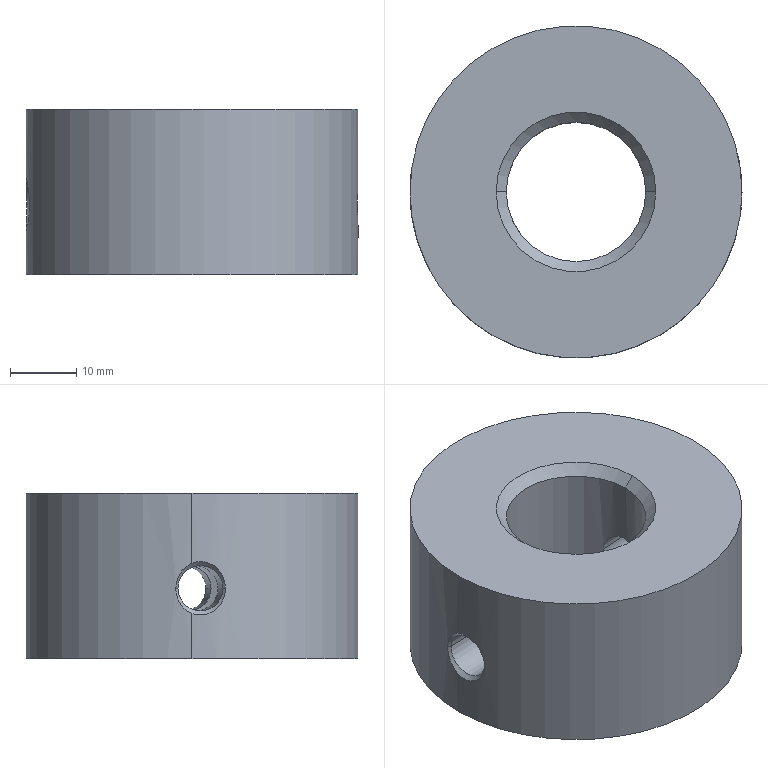Part | SolidWorks | features 3DProfileFeature 2, HoleWzd 2, Extrusion 1 | 1 solid | 14 faces | box 50 x 50 x 25 mm | volume 39286 mm3 | cylinder 8 | cone 4 | plane 2 | commonest cylinder face diameters 6.8 x4 21 x2 50 x2
STEP:
#1=CARTESIAN_POINT('',(24.555,4.697,10.643));
#2=VERTEX_POINT('',#1);
#3=CARTESIAN_POINT('',(25.,0.,7.507));
#4=VERTEX_POINT('',#3);
#5=CARTESIAN_POINT('',(24.555,4.697,10.643));
#6=CARTESIAN_POINT('',(24.555,4.697,10.365));
#7=CARTESIAN_POINT('',(24.561,4.663,10.087));
#8=CARTESIAN_POINT('',(24.587,4.527,9.543));
#9=CARTESIAN_POINT('',(24.605,4.428,9.284));
#10=CARTESIAN_POINT('',(24.639,4.232,8.916));
#11=CARTESIAN_POINT('',(24.652,4.158,8.796));
#12=CARTESIAN_POINT('',(24.678,3.999,8.568));
#13=CARTESIAN_POINT('',(24.692,3.913,8.46));
#14=CARTESIAN_POINT('',(24.735,3.635,8.152));
#15=CARTESIAN_POINT('',(24.766,3.421,7.967));
#16=CARTESIAN_POINT('',(24.825,2.961,7.659));
#17=CARTESIAN_POINT('',(24.854,2.715,7.535));
#18=CARTESIAN_POINT('',(24.906,2.186,7.346));
#19=CARTESIAN_POINT('',(24.928,1.916,7.286));
#20=CARTESIAN_POINT('',(24.964,1.363,7.232));
#21=CARTESIAN_POINT('',(24.978,1.079,7.24));
#22=CARTESIAN_POINT('',(24.991,0.6674,7.303));
#23=CARTESIAN_POINT('',(24.995,0.5315,7.332));
#24=CARTESIAN_POINT('',(24.999,0.2625,7.407));
#25=CARTESIAN_POINT('',(25.,0.1288,7.454));
#26=CARTESIAN_POINT('',(25.,0.,7.507));
#27=B_SPLINE_CURVE_WITH_KNOTS('',3,(#5,#6,#7,#8,#9,#10,#11,#12,#13,#14,#15,#16,#17,#18,#19,#20,#21,#22,#23,#24,#25,#26),.UNSPECIFIED.,.F.,.F.,(4,2,2,2,2,2,2,2,2,2,4),(0.01064,0.01148,0.01231,0.01272,0.01314,0.01397,0.01481,0.01564,0.01647,0.01689,0.01731),.UNSPECIFIED.);
#28=EDGE_CURVE('',#2,#4,#27,.T.);
#29=ORIENTED_EDGE('',*,*,#28,.F.);
#30=CARTESIAN_POINT('',(9.742,3.917,10.643));
#31=VERTEX_POINT('',#30);
#32=CARTESIAN_POINT('',(-25.144,2.082,10.643));
#33=DIRECTION('',(-0.9986,-0.05254,0.));
#34=VECTOR('',#33,1000.);
#35=LINE('',#32,#34);
#36=EDGE_CURVE('',#2,#31,#35,.T.);
#37=ORIENTED_EDGE('',*,*,#36,.T.);
#38=CARTESIAN_POINT('',(10.5,0.,7.288));
#39=VERTEX_POINT('',#38);
#40=CARTESIAN_POINT('',(10.5,0.,7.288));
#41=CARTESIAN_POINT('',(10.5,0.2463,7.248));
#42=CARTESIAN_POINT('',(10.491,0.4921,7.235));
#43=CARTESIAN_POINT('',(10.457,0.9829,7.262));
#44=CARTESIAN_POINT('',(10.43,1.23,7.303));
#45=CARTESIAN_POINT('',(10.364,1.7,7.436));
#46=CARTESIAN_POINT('',(10.324,1.926,7.527));
#47=CARTESIAN_POINT('',(10.234,2.358,7.759));
#48=CARTESIAN_POINT('',(10.186,2.557,7.896));
#49=CARTESIAN_POINT('',(10.087,2.923,8.212));
#50=CARTESIAN_POINT('',(10.036,3.091,8.392));
#51=CARTESIAN_POINT('',(9.942,3.381,8.779));
#52=CARTESIAN_POINT('',(9.899,3.504,8.987));
#53=CARTESIAN_POINT('',(9.824,3.709,9.435));
#54=CARTESIAN_POINT('',(9.794,3.786,9.668));
#55=CARTESIAN_POINT('',(9.753,3.89,10.147));
#56=CARTESIAN_POINT('',(9.742,3.917,10.397));
#57=CARTESIAN_POINT('',(9.742,3.917,10.643));
#58=B_SPLINE_CURVE_WITH_KNOTS('',3,(#40,#41,#42,#43,#44,#45,#46,#47,#48,#49,#50,#51,#52,#53,#54,#55,#56,#57),.UNSPECIFIED.,.F.,.F.,(4,2,2,2,2,2,2,2,4),(0.,0.0007379,0.001476,0.002214,0.002952,0.00369,0.004427,0.005165,0.005903),.UNSPECIFIED.);
#59=EDGE_CURVE('',#39,#31,#58,.T.);
#60=ORIENTED_EDGE('',*,*,#59,.F.);
#61=CARTESIAN_POINT('',(10.099,-2.873,10.643));
#62=VERTEX_POINT('',#61);
#63=CARTESIAN_POINT('',(10.099,-2.873,10.643));
#64=CARTESIAN_POINT('',(10.099,-2.873,10.443));
#65=CARTESIAN_POINT('',(10.105,-2.855,10.239));
#66=CARTESIAN_POINT('',(10.125,-2.783,9.845));
#67=CARTESIAN_POINT('',(10.139,-2.73,9.653));
#68=CARTESIAN_POINT('',(10.176,-2.589,9.277));
#69=CARTESIAN_POINT('',(10.198,-2.501,9.095));
#70=CARTESIAN_POINT('',(10.246,-2.298,8.753));
#71=CARTESIAN_POINT('',(10.272,-2.182,8.592));
#72=CARTESIAN_POINT('',(10.324,-1.92,8.288));
#73=CARTESIAN_POINT('',(10.35,-1.776,8.148));
#74=CARTESIAN_POINT('',(10.398,-1.469,7.897));
#75=CARTESIAN_POINT('',(10.42,-1.305,7.784));
#76=CARTESIAN_POINT('',(10.477,-0.7779,7.488));
#77=CARTESIAN_POINT('',(10.5,-0.4003,7.354));
#78=CARTESIAN_POINT('',(10.5,0.,7.288));
#79=B_SPLINE_CURVE_WITH_KNOTS('',3,(#63,#64,#65,#66,#67,#68,#69,#70,#71,#72,#73,#74,#75,#76,#77,#78),.UNSPECIFIED.,.F.,.F.,(4,2,2,2,2,2,2,4),(0.01661,0.01721,0.01781,0.01841,0.01901,0.01961,0.02021,0.02141),.UNSPECIFIED.);
#80=EDGE_CURVE('',#62,#39,#79,.T.);
#81=ORIENTED_EDGE('',*,*,#80,.F.);
#82=CARTESIAN_POINT('',(24.912,-2.094,10.643));
#83=VERTEX_POINT('',#82);
#84=CARTESIAN_POINT('',(-24.787,-4.709,10.643));
#85=DIRECTION('',(-0.9986,-0.05254,0.));
#86=VECTOR('',#85,1000.);
#87=LINE('',#84,#86);
#88=EDGE_CURVE('',#83,#62,#87,.T.);
#89=ORIENTED_EDGE('',*,*,#88,.F.);
#90=CARTESIAN_POINT('',(25.,0.,7.507));
#91=CARTESIAN_POINT('',(25.,-0.3073,7.636));
#92=CARTESIAN_POINT('',(24.994,-0.5936,7.808));
#93=CARTESIAN_POINT('',(24.977,-1.111,8.233));
#94=CARTESIAN_POINT('',(24.965,-1.333,8.479));
#95=CARTESIAN_POINT('',(24.942,-1.706,9.035));
#96=CARTESIAN_POINT('',(24.932,-1.849,9.336));
#97=CARTESIAN_POINT('',(24.92,-1.995,9.814));
#98=CARTESIAN_POINT('',(24.917,-2.032,9.978));
#99=CARTESIAN_POINT('',(24.913,-2.082,10.309));
#100=CARTESIAN_POINT('',(24.912,-2.094,10.475));
#101=CARTESIAN_POINT('',(24.912,-2.094,10.643));
#102=B_SPLINE_CURVE_WITH_KNOTS('',3,(#90,#91,#92,#93,#94,#95,#96,#97,#98,#99,#100,#101),.UNSPECIFIED.,.F.,.F.,(4,2,2,2,2,4),(0.01731,0.0183,0.01929,0.02029,0.02078,0.02128),.UNSPECIFIED.);
#103=EDGE_CURVE('',#4,#83,#102,.T.);
#104=ORIENTED_EDGE('',*,*,#103,.F.);
#105=EDGE_LOOP('',(#29,#37,#60,#81,#89,#104));
#106=FACE_OUTER_BOUND('',#105,.T.);
#107=CARTESIAN_POINT('',(-24.965,-1.314,10.643));
#108=DIRECTION('',(-0.9986,-0.05254,0.));
#109=DIRECTION('',(0.05254,-0.9986,0.));
#110=AXIS2_PLACEMENT_3D('',#107,#108,#109);
#111=CYLINDRICAL_SURFACE('',#110,3.4);
#112=ADVANCED_FACE('',(#106),#111,.F.);
#113=CARTESIAN_POINT('',(-10.099,2.873,10.643));
#114=VERTEX_POINT('',#113);
#115=CARTESIAN_POINT('',(-10.5,0.,7.288));
#116=VERTEX_POINT('',#115);
#117=CARTESIAN_POINT('',(-10.099,2.873,10.643));
#118=CARTESIAN_POINT('',(-10.099,2.873,10.244));
#119=CARTESIAN_POINT('',(-10.121,2.799,9.839));
#120=CARTESIAN_POINT('',(-10.176,2.589,9.278));
#121=CARTESIAN_POINT('',(-10.198,2.502,9.096));
#122=CARTESIAN_POINT('',(-10.246,2.297,8.752));
#123=CARTESIAN_POINT('',(-10.272,2.181,8.591));
#124=CARTESIAN_POINT('',(-10.324,1.921,8.289));
#125=CARTESIAN_POINT('',(-10.35,1.777,8.148));
#126=CARTESIAN_POINT('',(-10.398,1.467,7.895));
#127=CARTESIAN_POINT('',(-10.42,1.303,7.783));
#128=CARTESIAN_POINT('',(-10.458,0.9555,7.588));
#129=CARTESIAN_POINT('',(-10.473,0.7699,7.503));
#130=CARTESIAN_POINT('',(-10.494,0.3914,7.37));
#131=CARTESIAN_POINT('',(-10.5,0.1978,7.321));
#132=CARTESIAN_POINT('',(-10.5,0.,7.288));
#133=B_SPLINE_CURVE_WITH_KNOTS('',3,(#117,#118,#119,#120,#121,#122,#123,#124,#125,#126,#127,#128,#129,#130,#131,#132),.UNSPECIFIED.,.F.,.F.,(4,2,2,2,2,2,2,4),(0.0107,0.0119,0.0125,0.0131,0.0137,0.0143,0.0149,0.0155),.UNSPECIFIED.);
#134=EDGE_CURVE('',#114,#116,#133,.T.);
#135=ORIENTED_EDGE('',*,*,#134,.F.);
#136=CARTESIAN_POINT('',(-24.52,2.115,10.643));
#137=VERTEX_POINT('',#136);
#138=CARTESIAN_POINT('',(-25.144,2.082,10.643));
#139=DIRECTION('',(-0.9986,-0.05254,0.));
#140=VECTOR('',#139,1000.);
#141=LINE('',#138,#140);
#142=EDGE_CURVE('',#114,#137,#141,.T.);
#143=ORIENTED_EDGE('',*,*,#142,.T.);
#144=CARTESIAN_POINT('',(-24.163,-4.676,10.643));
#145=VERTEX_POINT('',#144);
#146=CARTESIAN_POINT('',(-24.341,-1.281,10.643));
#147=DIRECTION('',(-0.9986,-0.05254,0.));
#148=DIRECTION('',(0.05254,-0.9986,0.));
#149=AXIS2_PLACEMENT_3D('',#146,#147,#148);
#150=CIRCLE('',#149,3.4);
#151=EDGE_CURVE('',#137,#145,#150,.T.);
#152=ORIENTED_EDGE('',*,*,#151,.T.);
#153=CARTESIAN_POINT('',(-9.742,-3.917,10.643));
#154=VERTEX_POINT('',#153);
#155=CARTESIAN_POINT('',(-24.787,-4.709,10.643));
#156=DIRECTION('',(-0.9986,-0.05254,0.));
#157=VECTOR('',#156,1000.);
#158=LINE('',#155,#157);
#159=EDGE_CURVE('',#154,#145,#158,.T.);
#160=ORIENTED_EDGE('',*,*,#159,.F.);
#161=CARTESIAN_POINT('',(-10.5,0.,7.288));
#162=CARTESIAN_POINT('',(-10.5,-0.2432,7.249));
#163=CARTESIAN_POINT('',(-10.491,-0.4945,7.235));
#164=CARTESIAN_POINT('',(-10.457,-0.9847,7.262));
#165=CARTESIAN_POINT('',(-10.431,-1.228,7.303));
#166=CARTESIAN_POINT('',(-10.364,-1.703,7.436));
#167=CARTESIAN_POINT('',(-10.324,-1.928,7.528));
#168=CARTESIAN_POINT('',(-10.235,-2.355,7.758));
#169=CARTESIAN_POINT('',(-10.185,-2.558,7.897));
#170=CARTESIAN_POINT('',(-10.087,-2.924,8.213));
#171=CARTESIAN_POINT('',(-10.036,-3.089,8.39));
#172=CARTESIAN_POINT('',(-9.942,-3.382,8.781));
#173=CARTESIAN_POINT('',(-9.898,-3.505,8.989));
#174=CARTESIAN_POINT('',(-9.824,-3.708,9.432));
#175=CARTESIAN_POINT('',(-9.794,-3.787,9.669));
#176=CARTESIAN_POINT('',(-9.753,-3.891,10.149));
#177=CARTESIAN_POINT('',(-9.742,-3.917,10.394));
#178=CARTESIAN_POINT('',(-9.742,-3.917,10.643));
#179=B_SPLINE_CURVE_WITH_KNOTS('',3,(#161,#162,#163,#164,#165,#166,#167,#168,#169,#170,#171,#172,#173,#174,#175,#176,#177,#178),.UNSPECIFIED.,.F.,.F.,(4,2,2,2,2,2,2,2,4),(0.0155,0.01624,0.01698,0.01771,0.01845,0.01919,0.01993,0.02066,0.0214),.UNSPECIFIED.);
#180=EDGE_CURVE('',#116,#154,#179,.T.);
#181=ORIENTED_EDGE('',*,*,#180,.F.);
#182=EDGE_LOOP('',(#135,#143,#152,#160,#181));
#183=FACE_OUTER_BOUND('',#182,.T.);
#184=CARTESIAN_POINT('',(-24.965,-1.314,10.643));
#185=DIRECTION('',(-0.9986,-0.05254,0.));
#186=DIRECTION('',(0.05254,-0.9986,0.));
#187=AXIS2_PLACEMENT_3D('',#184,#185,#186);
#188=CYLINDRICAL_SURFACE('',#187,3.4);
#189=ADVANCED_FACE('',(#183),#188,.F.);
#190=ORIENTED_EDGE('',*,*,#151,.F.);
#191=CARTESIAN_POINT('',(-24.881,2.439,10.643));
#192=VERTEX_POINT('',#191);
#193=CARTESIAN_POINT('',(-25.177,2.706,10.643));
#194=DIRECTION('',(-0.7433,0.669,0.));
#195=VECTOR('',#194,1000.);
#196=LINE('',#193,#195);
#197=EDGE_CURVE('',#137,#192,#196,.T.);
#198=ORIENTED_EDGE('',*,*,#197,.T.);
#199=CARTESIAN_POINT('',(-25.,0.,6.875));
#200=VERTEX_POINT('',#199);
#201=CARTESIAN_POINT('',(-25.,0.,6.875));
#202=CARTESIAN_POINT('',(-25.,0.1848,6.95));
#203=CARTESIAN_POINT('',(-24.998,0.3615,7.039));
#204=CARTESIAN_POINT('',(-24.991,0.6998,7.245));
#205=CARTESIAN_POINT('',(-24.986,0.8625,7.363));
#206=CARTESIAN_POINT('',(-24.973,1.166,7.621));
#207=CARTESIAN_POINT('',(-24.966,1.306,7.76));
#208=CARTESIAN_POINT('',(-24.951,1.565,8.059));
#209=CARTESIAN_POINT('',(-24.943,1.684,8.22));
#210=CARTESIAN_POINT('',(-24.92,2.004,8.725));
#211=CARTESIAN_POINT('',(-24.906,2.165,9.085));
#212=CARTESIAN_POINT('',(-24.886,2.385,9.855));
#213=CARTESIAN_POINT('',(-24.881,2.439,10.246));
#214=CARTESIAN_POINT('',(-24.881,2.439,10.643));
#215=B_SPLINE_CURVE_WITH_KNOTS('',3,(#201,#202,#203,#204,#205,#206,#207,#208,#209,#210,#211,#212,#213,#214),.UNSPECIFIED.,.F.,.F.,(4,2,2,2,2,2,4),(0.003713,0.004306,0.004899,0.005493,0.006086,0.007273,0.00846),.UNSPECIFIED.);
#216=EDGE_CURVE('',#200,#192,#215,.T.);
#217=ORIENTED_EDGE('',*,*,#216,.F.);
#218=CARTESIAN_POINT('',(-24.487,-5.037,10.643));
#219=VERTEX_POINT('',#218);
#220=CARTESIAN_POINT('',(-24.487,-5.037,10.643));
#221=CARTESIAN_POINT('',(-24.487,-5.037,10.333));
#222=CARTESIAN_POINT('',(-24.494,-5.004,10.026));
#223=CARTESIAN_POINT('',(-24.514,-4.905,9.57));
#224=CARTESIAN_POINT('',(-24.522,-4.863,9.419));
#225=CARTESIAN_POINT('',(-24.542,-4.764,9.124));
#226=CARTESIAN_POINT('',(-24.553,-4.707,8.981));
#227=CARTESIAN_POINT('',(-24.577,-4.578,8.702));
#228=CARTESIAN_POINT('',(-24.591,-4.506,8.566));
#229=CARTESIAN_POINT('',(-24.62,-4.345,8.301));
#230=CARTESIAN_POINT('',(-24.635,-4.256,8.172));
#231=CARTESIAN_POINT('',(-24.683,-3.971,7.805));
#232=CARTESIAN_POINT('',(-24.718,-3.754,7.586));
#233=CARTESIAN_POINT('',(-24.787,-3.265,7.199));
#234=CARTESIAN_POINT('',(-24.821,-3.001,7.04));
#235=CARTESIAN_POINT('',(-24.867,-2.576,6.853));
#236=CARTESIAN_POINT('',(-24.882,-2.429,6.799));
#237=CARTESIAN_POINT('',(-24.909,-2.132,6.713));
#238=CARTESIAN_POINT('',(-24.922,-1.981,6.68));
#239=CARTESIAN_POINT('',(-24.955,-1.524,6.611));
#240=CARTESIAN_POINT('',(-24.973,-1.208,6.606));
#241=CARTESIAN_POINT('',(-24.989,-0.7464,6.662));
#242=CARTESIAN_POINT('',(-24.993,-0.5945,6.69));
#243=CARTESIAN_POINT('',(-24.999,-0.2941,6.768));
#244=CARTESIAN_POINT('',(-25.,-0.1446,6.817));
#245=CARTESIAN_POINT('',(-25.,0.,6.875));
#246=B_SPLINE_CURVE_WITH_KNOTS('',3,(#220,#221,#222,#223,#224,#225,#226,#227,#228,#229,#230,#231,#232,#233,#234,#235,#236,#237,#238,#239,#240,#241,#242,#243,#244,#245),.UNSPECIFIED.,.F.,.F.,(4,2,2,2,2,2,2,2,2,2,2,2,4),(0.02064,0.02157,0.02203,0.0225,0.02296,0.02343,0.02435,0.02528,0.02575,0.02621,0.02714,0.02761,0.02807),.UNSPECIFIED.);
#247=EDGE_CURVE('',#219,#200,#246,.T.);
#248=ORIENTED_EDGE('',*,*,#247,.F.);
#249=CARTESIAN_POINT('',(-24.754,-5.333,10.643));
#250=DIRECTION('',(-0.669,-0.7433,0.));
#251=VECTOR('',#250,1000.);
#252=LINE('',#249,#251);
#253=EDGE_CURVE('',#145,#219,#252,.T.);
#254=ORIENTED_EDGE('',*,*,#253,.F.);
#255=EDGE_LOOP('',(#190,#198,#217,#248,#254));
#256=FACE_OUTER_BOUND('',#255,.T.);
#257=CARTESIAN_POINT('',(-24.965,-1.314,10.643));
#258=DIRECTION('',(-0.9986,-0.05254,0.));
#259=DIRECTION('',(0.05254,-0.9986,0.));
#260=AXIS2_PLACEMENT_3D('',#257,#258,#259);
#261=CONICAL_SURFACE('',#260,4.025,0.7854);
#262=ADVANCED_FACE('',(#256),#261,.F.);
#263=CARTESIAN_POINT('',(-10.5,0.,23.475));
#264=VERTEX_POINT('',#263);
#265=CARTESIAN_POINT('',(10.5,0.,23.475));
#266=VERTEX_POINT('',#265);
#267=CARTESIAN_POINT('',(0.,0.,23.475));
#268=DIRECTION('',(0.,0.,1.));
#269=DIRECTION('',(1.,0.,0.));
#270=AXIS2_PLACEMENT_3D('',#267,#268,#269);
#271=CIRCLE('',#270,10.5);
#272=EDGE_CURVE('',#264,#266,#271,.T.);
#273=ORIENTED_EDGE('',*,*,#272,.F.);
#274=CARTESIAN_POINT('',(-12.025,0.,25.));
#275=VERTEX_POINT('',#274);
#276=CARTESIAN_POINT('',(-12.025,0.,25.));
#277=DIRECTION('',(-0.7071,0.,0.7071));
#278=VECTOR('',#277,1000.);
#279=LINE('',#276,#278);
#280=EDGE_CURVE('',#264,#275,#279,.T.);
#281=ORIENTED_EDGE('',*,*,#280,.T.);
#282=CARTESIAN_POINT('',(12.025,0.,25.));
#283=VERTEX_POINT('',#282);
#284=CARTESIAN_POINT('',(0.,0.,25.));
#285=DIRECTION('',(0.,0.,1.));
#286=DIRECTION('',(1.,0.,0.));
#287=AXIS2_PLACEMENT_3D('',#284,#285,#286);
#288=CIRCLE('',#287,12.025);
#289=EDGE_CURVE('',#275,#283,#288,.T.);
#290=ORIENTED_EDGE('',*,*,#289,.T.);
#291=CARTESIAN_POINT('',(12.025,0.,25.));
#292=DIRECTION('',(0.7071,0.,0.7071));
#293=VECTOR('',#292,1000.);
#294=LINE('',#291,#293);
#295=EDGE_CURVE('',#266,#283,#294,.T.);
#296=ORIENTED_EDGE('',*,*,#295,.F.);
#297=EDGE_LOOP('',(#273,#281,#290,#296));
#298=FACE_OUTER_BOUND('',#297,.T.);
#299=CARTESIAN_POINT('',(0.,0.,25.));
#300=DIRECTION('',(0.,0.,1.));
#301=DIRECTION('',(1.,0.,0.));
#302=AXIS2_PLACEMENT_3D('',#299,#300,#301);
#303=CONICAL_SURFACE('',#302,12.025,0.7854);
#304=ADVANCED_FACE('',(#298),#303,.F.);
#305=CARTESIAN_POINT('',(-10.5,0.,0.));
#306=VERTEX_POINT('',#305);
#307=CARTESIAN_POINT('',(10.5,0.,0.));
#308=VERTEX_POINT('',#307);
#309=CARTESIAN_POINT('',(0.,0.,0.));
#310=DIRECTION('',(0.,0.,1.));
#311=DIRECTION('',(1.,0.,0.));
#312=AXIS2_PLACEMENT_3D('',#309,#310,#311);
#313=CIRCLE('',#312,10.5);
#314=EDGE_CURVE('',#306,#308,#313,.T.);
#315=ORIENTED_EDGE('',*,*,#314,.F.);
#316=CARTESIAN_POINT('',(-10.5,0.,25.));
#317=DIRECTION('',(0.,0.,1.));
#318=VECTOR('',#317,1000.);
#319=LINE('',#316,#318);
#320=EDGE_CURVE('',#306,#116,#319,.T.);
#321=ORIENTED_EDGE('',*,*,#320,.T.);
#322=ORIENTED_EDGE('',*,*,#180,.T.);
#323=CARTESIAN_POINT('',(-10.5,0.,13.998));
#324=VERTEX_POINT('',#323);
#325=CARTESIAN_POINT('',(-9.742,-3.917,10.643));
#326=CARTESIAN_POINT('',(-9.742,-3.917,10.893));
#327=CARTESIAN_POINT('',(-9.753,-3.891,11.138));
#328=CARTESIAN_POINT('',(-9.794,-3.787,11.617));
#329=CARTESIAN_POINT('',(-9.824,-3.708,11.855));
#330=CARTESIAN_POINT('',(-9.898,-3.505,12.298));
#331=CARTESIAN_POINT('',(-9.942,-3.382,12.507));
#332=CARTESIAN_POINT('',(-10.037,-3.088,12.899));
#333=CARTESIAN_POINT('',(-10.087,-2.923,13.075));
#334=CARTESIAN_POINT('',(-10.186,-2.557,13.39));
#335=CARTESIAN_POINT('',(-10.235,-2.354,13.53));
#336=CARTESIAN_POINT('',(-10.324,-1.927,13.759));
#337=CARTESIAN_POINT('',(-10.364,-1.702,13.851));
#338=CARTESIAN_POINT('',(-10.431,-1.229,13.984));
#339=CARTESIAN_POINT('',(-10.457,-0.9844,14.025));
#340=CARTESIAN_POINT('',(-10.491,-0.4947,14.052));
#341=CARTESIAN_POINT('',(-10.5,-0.2439,14.038));
#342=CARTESIAN_POINT('',(-10.5,0.,13.998));
#343=B_SPLINE_CURVE_WITH_KNOTS('',3,(#325,#326,#327,#328,#329,#330,#331,#332,#333,#334,#335,#336,#337,#338,#339,#340,#341,#342),.UNSPECIFIED.,.F.,.F.,(4,2,2,2,2,2,2,2,4),(0.,0.0007378,0.001476,0.002213,0.002951,0.003689,0.004427,0.005165,0.005902),.UNSPECIFIED.);
#344=EDGE_CURVE('',#154,#324,#343,.T.);
#345=ORIENTED_EDGE('',*,*,#344,.T.);
#346=CARTESIAN_POINT('',(-10.5,0.,25.));
#347=DIRECTION('',(0.,0.,1.));
#348=VECTOR('',#347,1000.);
#349=LINE('',#346,#348);
#350=EDGE_CURVE('',#324,#264,#349,.T.);
#351=ORIENTED_EDGE('',*,*,#350,.T.);
#352=ORIENTED_EDGE('',*,*,#272,.T.);
#353=CARTESIAN_POINT('',(10.5,0.,13.998));
#354=VERTEX_POINT('',#353);
#355=CARTESIAN_POINT('',(10.5,0.,25.));
#356=DIRECTION('',(0.,0.,1.));
#357=VECTOR('',#356,1000.);
#358=LINE('',#355,#357);
#359=EDGE_CURVE('',#354,#266,#358,.T.);
#360=ORIENTED_EDGE('',*,*,#359,.F.);
#361=CARTESIAN_POINT('',(10.5,0.,13.998));
#362=CARTESIAN_POINT('',(10.5,-0.1975,13.966));
#363=CARTESIAN_POINT('',(10.494,-0.3929,13.916));
#364=CARTESIAN_POINT('',(10.473,-0.7744,13.782));
#365=CARTESIAN_POINT('',(10.458,-0.9564,13.699));
#366=CARTESIAN_POINT('',(10.42,-1.304,13.503));
#367=CARTESIAN_POINT('',(10.398,-1.471,13.389));
#368=CARTESIAN_POINT('',(10.349,-1.781,13.135));
#369=CARTESIAN_POINT('',(10.323,-1.923,12.996));
#370=CARTESIAN_POINT('',(10.272,-2.182,12.695));
#371=CARTESIAN_POINT('',(10.246,-2.3,12.531));
#372=CARTESIAN_POINT('',(10.198,-2.504,12.187));
#373=CARTESIAN_POINT('',(10.176,-2.589,12.008));
#374=CARTESIAN_POINT('',(10.139,-2.729,11.634));
#375=CARTESIAN_POINT('',(10.124,-2.784,11.438));
#376=CARTESIAN_POINT('',(10.104,-2.855,11.043));
#377=CARTESIAN_POINT('',(10.099,-2.873,10.844));
#378=CARTESIAN_POINT('',(10.099,-2.873,10.643));
#379=B_SPLINE_CURVE_WITH_KNOTS('',3,(#361,#362,#363,#364,#365,#366,#367,#368,#369,#370,#371,#372,#373,#374,#375,#376,#377,#378),.UNSPECIFIED.,.F.,.F.,(4,2,2,2,2,2,2,2,4),(0.01181,0.01241,0.01301,0.01361,0.01421,0.01481,0.01541,0.01601,0.01661),.UNSPECIFIED.);
#380=EDGE_CURVE('',#354,#62,#379,.T.);
#381=ORIENTED_EDGE('',*,*,#380,.T.);
#382=ORIENTED_EDGE('',*,*,#80,.T.);
#383=CARTESIAN_POINT('',(10.5,0.,25.));
#384=DIRECTION('',(0.,0.,1.));
#385=VECTOR('',#384,1000.);
#386=LINE('',#383,#385);
#387=EDGE_CURVE('',#308,#39,#386,.T.);
#388=ORIENTED_EDGE('',*,*,#387,.F.);
#389=EDGE_LOOP('',(#315,#321,#322,#345,#351,#352,#360,#381,#382,#388));
#390=FACE_OUTER_BOUND('',#389,.T.);
#391=CARTESIAN_POINT('',(0.,0.,25.));
#392=DIRECTION('',(0.,0.,1.));
#393=DIRECTION('',(1.,0.,0.));
#394=AXIS2_PLACEMENT_3D('',#391,#392,#393);
#395=CYLINDRICAL_SURFACE('',#394,10.5);
#396=ADVANCED_FACE('',(#390),#395,.F.);
#397=CARTESIAN_POINT('',(25.,0.,25.));
#398=VERTEX_POINT('',#397);
#399=CARTESIAN_POINT('',(-25.,0.,25.));
#400=VERTEX_POINT('',#399);
#401=CARTESIAN_POINT('',(0.,0.,25.));
#402=DIRECTION('',(0.,0.,1.));
#403=DIRECTION('',(1.,0.,0.));
#404=AXIS2_PLACEMENT_3D('',#401,#402,#403);
#405=CIRCLE('',#404,25.);
#406=EDGE_CURVE('',#398,#400,#405,.T.);
#407=ORIENTED_EDGE('',*,*,#406,.F.);
#408=CARTESIAN_POINT('',(25.,0.,13.779));
#409=VERTEX_POINT('',#408);
#410=CARTESIAN_POINT('',(25.,0.,25.));
#411=DIRECTION('',(0.,0.,-1.));
#412=VECTOR('',#411,1000.);
#413=LINE('',#410,#412);
#414=EDGE_CURVE('',#398,#409,#413,.T.);
#415=ORIENTED_EDGE('',*,*,#414,.T.);
#416=CARTESIAN_POINT('',(25.,0.,13.779));
#417=CARTESIAN_POINT('',(25.,0.1281,13.833));
#418=CARTESIAN_POINT('',(24.999,0.2593,13.879));
#419=CARTESIAN_POINT('',(24.995,0.5285,13.954));
#420=CARTESIAN_POINT('',(24.991,0.6668,13.984));
#421=CARTESIAN_POINT('',(24.978,1.08,14.047));
#422=CARTESIAN_POINT('',(24.965,1.357,14.055));
#423=CARTESIAN_POINT('',(24.928,1.916,14.001));
#424=CARTESIAN_POINT('',(24.905,2.187,13.94));
#425=CARTESIAN_POINT('',(24.854,2.709,13.754));
#426=CARTESIAN_POINT('',(24.825,2.962,13.627));
#427=CARTESIAN_POINT('',(24.781,3.306,13.397));
#428=CARTESIAN_POINT('',(24.766,3.416,13.313));
#429=CARTESIAN_POINT('',(24.736,3.626,13.131));
#430=CARTESIAN_POINT('',(24.721,3.727,13.033));
#431=CARTESIAN_POINT('',(24.678,4.006,12.723));
#432=CARTESIAN_POINT('',(24.651,4.165,12.497));
#433=CARTESIAN_POINT('',(24.617,4.361,12.128));
#434=CARTESIAN_POINT('',(24.606,4.42,12.));
#435=CARTESIAN_POINT('',(24.588,4.519,11.74));
#436=CARTESIAN_POINT('',(24.58,4.561,11.608));
#437=CARTESIAN_POINT('',(24.562,4.662,11.204));
#438=CARTESIAN_POINT('',(24.555,4.697,10.921));
#439=CARTESIAN_POINT('',(24.555,4.697,10.643));
#440=B_SPLINE_CURVE_WITH_KNOTS('',3,(#416,#417,#418,#419,#420,#421,#422,#423,#424,#425,#426,#427,#428,#429,#430,#431,#432,#433,#434,#435,#436,#437,#438,#439),.UNSPECIFIED.,.F.,.F.,(4,2,2,2,2,2,2,2,2,2,2,4),(0.003979,0.004395,0.004812,0.005645,0.006478,0.00731,0.007727,0.008143,0.008976,0.009393,0.009809,0.01064),.UNSPECIFIED.);
#441=EDGE_CURVE('',#409,#2,#440,.T.);
#442=ORIENTED_EDGE('',*,*,#441,.T.);
#443=ORIENTED_EDGE('',*,*,#28,.T.);
#444=CARTESIAN_POINT('',(25.,0.,0.));
#445=VERTEX_POINT('',#444);
#446=CARTESIAN_POINT('',(25.,0.,25.));
#447=DIRECTION('',(0.,0.,-1.));
#448=VECTOR('',#447,1000.);
#449=LINE('',#446,#448);
#450=EDGE_CURVE('',#4,#445,#449,.T.);
#451=ORIENTED_EDGE('',*,*,#450,.T.);
#452=CARTESIAN_POINT('',(-25.,0.,0.));
#453=VERTEX_POINT('',#452);
#454=CARTESIAN_POINT('',(0.,0.,0.));
#455=DIRECTION('',(0.,0.,1.));
#456=DIRECTION('',(1.,0.,0.));
#457=AXIS2_PLACEMENT_3D('',#454,#455,#456);
#458=CIRCLE('',#457,25.);
#459=EDGE_CURVE('',#445,#453,#458,.T.);
#460=ORIENTED_EDGE('',*,*,#459,.T.);
#461=CARTESIAN_POINT('',(-25.,0.,25.));
#462=DIRECTION('',(0.,0.,-1.));
#463=VECTOR('',#462,1000.);
#464=LINE('',#461,#463);
#465=EDGE_CURVE('',#200,#453,#464,.T.);
#466=ORIENTED_EDGE('',*,*,#465,.F.);
#467=ORIENTED_EDGE('',*,*,#216,.T.);
#468=CARTESIAN_POINT('',(-25.,0.,14.412));
#469=VERTEX_POINT('',#468);
#470=CARTESIAN_POINT('',(-24.881,2.439,10.643));
#471=CARTESIAN_POINT('',(-24.881,2.439,10.842));
#472=CARTESIAN_POINT('',(-24.882,2.425,11.043));
#473=CARTESIAN_POINT('',(-24.887,2.37,11.435));
#474=CARTESIAN_POINT('',(-24.891,2.329,11.628));
#475=CARTESIAN_POINT('',(-24.901,2.22,12.008));
#476=CARTESIAN_POINT('',(-24.907,2.152,12.197));
#477=CARTESIAN_POINT('',(-24.921,1.989,12.56));
#478=CARTESIAN_POINT('',(-24.928,1.895,12.734));
#479=CARTESIAN_POINT('',(-24.943,1.684,13.067));
#480=CARTESIAN_POINT('',(-24.951,1.566,13.226));
#481=CARTESIAN_POINT('',(-24.966,1.305,13.528));
#482=CARTESIAN_POINT('',(-24.973,1.163,13.668));
#483=CARTESIAN_POINT('',(-24.986,0.8624,13.924));
#484=CARTESIAN_POINT('',(-24.991,0.7028,14.04));
#485=CARTESIAN_POINT('',(-24.998,0.3643,14.246));
#486=CARTESIAN_POINT('',(-25.,0.1838,14.337));
#487=CARTESIAN_POINT('',(-25.,0.,14.412));
#488=B_SPLINE_CURVE_WITH_KNOTS('',3,(#470,#471,#472,#473,#474,#475,#476,#477,#478,#479,#480,#481,#482,#483,#484,#485,#486,#487),.UNSPECIFIED.,.F.,.F.,(4,2,2,2,2,2,2,2,4),(0.00846,0.009054,0.009648,0.01024,0.01084,0.01143,0.01202,0.01262,0.01321),.UNSPECIFIED.);
#489=EDGE_CURVE('',#192,#469,#488,.T.);
#490=ORIENTED_EDGE('',*,*,#489,.T.);
#491=CARTESIAN_POINT('',(-25.,0.,25.));
#492=DIRECTION('',(0.,0.,-1.));
#493=VECTOR('',#492,1000.);
#494=LINE('',#491,#493);
#495=EDGE_CURVE('',#400,#469,#494,.T.);
#496=ORIENTED_EDGE('',*,*,#495,.F.);
#497=EDGE_LOOP('',(#407,#415,#442,#443,#451,#460,#466,#467,#490,#496));
#498=FACE_OUTER_BOUND('',#497,.T.);
#499=CARTESIAN_POINT('',(0.,0.,25.));
#500=DIRECTION('',(0.,0.,-1.));
#501=DIRECTION('',(-1.,0.,0.));
#502=AXIS2_PLACEMENT_3D('',#499,#500,#501);
#503=CYLINDRICAL_SURFACE('',#502,25.);
#504=ADVANCED_FACE('',(#498),#503,.T.);
#505=ORIENTED_EDGE('',*,*,#414,.F.);
#506=CARTESIAN_POINT('',(0.,0.,25.));
#507=DIRECTION('',(0.,0.,1.));
#508=DIRECTION('',(1.,0.,0.));
#509=AXIS2_PLACEMENT_3D('',#506,#507,#508);
#510=CIRCLE('',#509,25.);
#511=EDGE_CURVE('',#400,#398,#510,.T.);
#512=ORIENTED_EDGE('',*,*,#511,.F.);
#513=ORIENTED_EDGE('',*,*,#495,.T.);
#514=CARTESIAN_POINT('',(-25.,0.,14.412));
#515=CARTESIAN_POINT('',(-25.,-0.2874,14.528));
#516=CARTESIAN_POINT('',(-24.995,-0.5861,14.606));
#517=CARTESIAN_POINT('',(-24.973,-1.207,14.681));
#518=CARTESIAN_POINT('',(-24.956,-1.518,14.676));
#519=CARTESIAN_POINT('',(-24.922,-1.977,14.608));
#520=CARTESIAN_POINT('',(-24.91,-2.13,14.574));
#521=CARTESIAN_POINT('',(-24.882,-2.429,14.488));
#522=CARTESIAN_POINT('',(-24.868,-2.574,14.435));
#523=CARTESIAN_POINT('',(-24.821,-2.997,14.249));
#524=CARTESIAN_POINT('',(-24.787,-3.266,14.086));
#525=CARTESIAN_POINT('',(-24.718,-3.75,13.705));
#526=CARTESIAN_POINT('',(-24.684,-3.969,13.483));
#527=CARTESIAN_POINT('',(-24.619,-4.35,12.994));
#528=CARTESIAN_POINT('',(-24.59,-4.51,12.731));
#529=CARTESIAN_POINT('',(-24.553,-4.706,12.309));
#530=CARTESIAN_POINT('',(-24.542,-4.764,12.163));
#531=CARTESIAN_POINT('',(-24.523,-4.863,11.869));
#532=CARTESIAN_POINT('',(-24.514,-4.904,11.72));
#533=CARTESIAN_POINT('',(-24.501,-4.97,11.418));
#534=CARTESIAN_POINT('',(-24.496,-4.995,11.265));
#535=CARTESIAN_POINT('',(-24.489,-5.028,10.956));
#536=CARTESIAN_POINT('',(-24.487,-5.037,10.799));
#537=CARTESIAN_POINT('',(-24.487,-5.037,10.643));
#538=B_SPLINE_CURVE_WITH_KNOTS('',3,(#514,#515,#516,#517,#518,#519,#520,#521,#522,#523,#524,#525,#526,#527,#528,#529,#530,#531,#532,#533,#534,#535,#536,#537),.UNSPECIFIED.,.F.,.F.,(4,2,2,2,2,2,2,2,2,2,2,4),(0.01321,0.01414,0.01507,0.01553,0.016,0.01693,0.01785,0.01878,0.01925,0.01971,0.02018,0.02064),.UNSPECIFIED.);
#539=EDGE_CURVE('',#469,#219,#538,.T.);
#540=ORIENTED_EDGE('',*,*,#539,.T.);
#541=ORIENTED_EDGE('',*,*,#247,.T.);
#542=ORIENTED_EDGE('',*,*,#465,.T.);
#543=CARTESIAN_POINT('',(0.,0.,0.));
#544=DIRECTION('',(0.,0.,1.));
#545=DIRECTION('',(1.,0.,0.));
#546=AXIS2_PLACEMENT_3D('',#543,#544,#545);
#547=CIRCLE('',#546,25.);
#548=EDGE_CURVE('',#453,#445,#547,.T.);
#549=ORIENTED_EDGE('',*,*,#548,.T.);
#550=ORIENTED_EDGE('',*,*,#450,.F.);
#551=ORIENTED_EDGE('',*,*,#103,.T.);
#552=CARTESIAN_POINT('',(24.912,-2.094,10.643));
#553=CARTESIAN_POINT('',(24.912,-2.094,10.98));
#554=CARTESIAN_POINT('',(24.916,-2.045,11.308));
#555=CARTESIAN_POINT('',(24.928,-1.899,11.787));
#556=CARTESIAN_POINT('',(24.932,-1.838,11.945));
#557=CARTESIAN_POINT('',(24.943,-1.696,12.245));
#558=CARTESIAN_POINT('',(24.948,-1.614,12.389));
#559=CARTESIAN_POINT('',(24.959,-1.429,12.665));
#560=CARTESIAN_POINT('',(24.965,-1.325,12.798));
#561=CARTESIAN_POINT('',(24.976,-1.101,13.045));
#562=CARTESIAN_POINT('',(24.981,-0.9814,13.16));
#563=CARTESIAN_POINT('',(24.994,-0.5972,13.476));
#564=CARTESIAN_POINT('',(25.,-0.3058,13.652));
#565=CARTESIAN_POINT('',(25.,0.,13.779));
#566=B_SPLINE_CURVE_WITH_KNOTS('',3,(#552,#553,#554,#555,#556,#557,#558,#559,#560,#561,#562,#563,#564,#565),.UNSPECIFIED.,.F.,.F.,(4,2,2,2,2,2,4),(0.,0.0009947,0.001492,0.001989,0.002487,0.002984,0.003979),.UNSPECIFIED.);
#567=EDGE_CURVE('',#83,#409,#566,.T.);
#568=ORIENTED_EDGE('',*,*,#567,.T.);
#569=EDGE_LOOP('',(#505,#512,#513,#540,#541,#542,#549,#550,#551,#568));
#570=FACE_OUTER_BOUND('',#569,.T.);
#571=CARTESIAN_POINT('',(0.,0.,25.));
#572=DIRECTION('',(0.,0.,-1.));
#573=DIRECTION('',(-1.,0.,0.));
#574=AXIS2_PLACEMENT_3D('',#571,#572,#573);
#575=CYLINDRICAL_SURFACE('',#574,25.);
#576=ADVANCED_FACE('',(#570),#575,.T.);
#577=CARTESIAN_POINT('',(0.,0.,25.));
#578=DIRECTION('',(0.,0.,1.));
#579=DIRECTION('',(1.,0.,0.));
#580=AXIS2_PLACEMENT_3D('',#577,#578,#579);
#581=CIRCLE('',#580,12.025);
#582=EDGE_CURVE('',#283,#275,#581,.T.);
#583=ORIENTED_EDGE('',*,*,#582,.F.);
#584=ORIENTED_EDGE('',*,*,#289,.F.);
#585=EDGE_LOOP('',(#583,#584));
#586=FACE_BOUND('',#585,.T.);
#587=ORIENTED_EDGE('',*,*,#511,.T.);
#588=ORIENTED_EDGE('',*,*,#406,.T.);
#589=EDGE_LOOP('',(#587,#588));
#590=FACE_OUTER_BOUND('',#589,.T.);
#591=CARTESIAN_POINT('',(0.,0.,25.));
#592=DIRECTION('',(0.,0.,1.));
#593=DIRECTION('',(1.,0.,0.));
#594=AXIS2_PLACEMENT_3D('',#591,#592,#593);
#595=PLANE('',#594);
#596=ADVANCED_FACE('',(#586,#590),#595,.T.);
#597=CARTESIAN_POINT('',(0.,0.,0.));
#598=DIRECTION('',(0.,0.,1.));
#599=DIRECTION('',(1.,0.,0.));
#600=AXIS2_PLACEMENT_3D('',#597,#598,#599);
#601=CIRCLE('',#600,10.5);
#602=EDGE_CURVE('',#308,#306,#601,.T.);
#603=ORIENTED_EDGE('',*,*,#602,.T.);
#604=ORIENTED_EDGE('',*,*,#314,.T.);
#605=EDGE_LOOP('',(#603,#604));
#606=FACE_BOUND('',#605,.T.);
#607=ORIENTED_EDGE('',*,*,#548,.F.);
#608=ORIENTED_EDGE('',*,*,#459,.F.);
#609=EDGE_LOOP('',(#607,#608));
#610=FACE_OUTER_BOUND('',#609,.T.);
#611=CARTESIAN_POINT('',(0.,0.,0.));
#612=DIRECTION('',(0.,0.,1.));
#613=DIRECTION('',(1.,0.,0.));
#614=AXIS2_PLACEMENT_3D('',#611,#612,#613);
#615=PLANE('',#614);
#616=ADVANCED_FACE('',(#606,#610),#615,.F.);
#617=ORIENTED_EDGE('',*,*,#320,.F.);
#618=ORIENTED_EDGE('',*,*,#602,.F.);
#619=ORIENTED_EDGE('',*,*,#387,.T.);
#620=ORIENTED_EDGE('',*,*,#59,.T.);
#621=CARTESIAN_POINT('',(9.742,3.917,10.643));
#622=CARTESIAN_POINT('',(9.742,3.917,10.89));
#623=CARTESIAN_POINT('',(9.753,3.891,11.135));
#624=CARTESIAN_POINT('',(9.794,3.786,11.619));
#625=CARTESIAN_POINT('',(9.824,3.708,11.853));
#626=CARTESIAN_POINT('',(9.898,3.506,12.297));
#627=CARTESIAN_POINT('',(9.942,3.38,12.509));
#628=CARTESIAN_POINT('',(10.037,3.089,12.897));
#629=CARTESIAN_POINT('',(10.086,2.924,13.074));
#630=CARTESIAN_POINT('',(10.186,2.555,13.392));
#631=CARTESIAN_POINT('',(10.235,2.355,13.53));
#632=CARTESIAN_POINT('',(10.324,1.929,13.759));
#633=CARTESIAN_POINT('',(10.364,1.699,13.852));
#634=CARTESIAN_POINT('',(10.431,1.227,13.984));
#635=CARTESIAN_POINT('',(10.457,0.9861,14.025));
#636=CARTESIAN_POINT('',(10.491,0.4932,14.052));
#637=CARTESIAN_POINT('',(10.5,0.2428,14.038));
#638=CARTESIAN_POINT('',(10.5,0.,13.998));
#639=B_SPLINE_CURVE_WITH_KNOTS('',3,(#621,#622,#623,#624,#625,#626,#627,#628,#629,#630,#631,#632,#633,#634,#635,#636,#637,#638),.UNSPECIFIED.,.F.,.F.,(4,2,2,2,2,2,2,2,4),(0.005903,0.006641,0.00738,0.008118,0.008856,0.009594,0.01033,0.01107,0.01181),.UNSPECIFIED.);
#640=EDGE_CURVE('',#31,#354,#639,.T.);
#641=ORIENTED_EDGE('',*,*,#640,.T.);
#642=ORIENTED_EDGE('',*,*,#359,.T.);
#643=CARTESIAN_POINT('',(0.,0.,23.475));
#644=DIRECTION('',(0.,0.,1.));
#645=DIRECTION('',(1.,0.,0.));
#646=AXIS2_PLACEMENT_3D('',#643,#644,#645);
#647=CIRCLE('',#646,10.5);
#648=EDGE_CURVE('',#266,#264,#647,.T.);
#649=ORIENTED_EDGE('',*,*,#648,.T.);
#650=ORIENTED_EDGE('',*,*,#350,.F.);
#651=CARTESIAN_POINT('',(-10.5,0.,13.998));
#652=CARTESIAN_POINT('',(-10.5,0.1984,13.966));
#653=CARTESIAN_POINT('',(-10.494,0.3922,13.916));
#654=CARTESIAN_POINT('',(-10.473,0.7709,13.783));
#655=CARTESIAN_POINT('',(-10.458,0.9564,13.699));
#656=CARTESIAN_POINT('',(-10.42,1.304,13.503));
#657=CARTESIAN_POINT('',(-10.398,1.469,13.391));
#658=CARTESIAN_POINT('',(-10.349,1.779,13.137));
#659=CARTESIAN_POINT('',(-10.323,1.923,12.996));
#660=CARTESIAN_POINT('',(-10.272,2.182,12.695));
#661=CARTESIAN_POINT('',(-10.246,2.298,12.534));
#662=CARTESIAN_POINT('',(-10.198,2.503,12.189));
#663=CARTESIAN_POINT('',(-10.176,2.59,12.007));
#664=CARTESIAN_POINT('',(-10.139,2.729,11.635));
#665=CARTESIAN_POINT('',(-10.125,2.783,11.442));
#666=CARTESIAN_POINT('',(-10.104,2.855,11.045));
#667=CARTESIAN_POINT('',(-10.099,2.873,10.843));
#668=CARTESIAN_POINT('',(-10.099,2.873,10.643));
#669=B_SPLINE_CURVE_WITH_KNOTS('',3,(#651,#652,#653,#654,#655,#656,#657,#658,#659,#660,#661,#662,#663,#664,#665,#666,#667,#668),.UNSPECIFIED.,.F.,.F.,(4,2,2,2,2,2,2,2,4),(0.005902,0.006502,0.007102,0.007702,0.008302,0.008902,0.009502,0.0101,0.0107),.UNSPECIFIED.);
#670=EDGE_CURVE('',#324,#114,#669,.T.);
#671=ORIENTED_EDGE('',*,*,#670,.T.);
#672=ORIENTED_EDGE('',*,*,#134,.T.);
#673=EDGE_LOOP('',(#617,#618,#619,#620,#641,#642,#649,#650,#671,#672));
#674=FACE_OUTER_BOUND('',#673,.T.);
#675=CARTESIAN_POINT('',(0.,0.,25.));
#676=DIRECTION('',(0.,0.,1.));
#677=DIRECTION('',(1.,0.,0.));
#678=AXIS2_PLACEMENT_3D('',#675,#676,#677);
#679=CYLINDRICAL_SURFACE('',#678,10.5);
#680=ADVANCED_FACE('',(#674),#679,.F.);
#681=ORIENTED_EDGE('',*,*,#280,.F.);
#682=ORIENTED_EDGE('',*,*,#648,.F.);
#683=ORIENTED_EDGE('',*,*,#295,.T.);
#684=ORIENTED_EDGE('',*,*,#582,.T.);
#685=EDGE_LOOP('',(#681,#682,#683,#684));
#686=FACE_OUTER_BOUND('',#685,.T.);
#687=CARTESIAN_POINT('',(0.,0.,25.));
#688=DIRECTION('',(0.,0.,1.));
#689=DIRECTION('',(1.,0.,0.));
#690=AXIS2_PLACEMENT_3D('',#687,#688,#689);
#691=CONICAL_SURFACE('',#690,12.025,0.7854);
#692=ADVANCED_FACE('',(#686),#691,.F.);
#693=ORIENTED_EDGE('',*,*,#197,.F.);
#694=CARTESIAN_POINT('',(-24.341,-1.281,10.643));
#695=DIRECTION('',(-0.9986,-0.05254,0.));
#696=DIRECTION('',(0.05254,-0.9986,0.));
#697=AXIS2_PLACEMENT_3D('',#694,#695,#696);
#698=CIRCLE('',#697,3.4);
#699=EDGE_CURVE('',#145,#137,#698,.T.);
#700=ORIENTED_EDGE('',*,*,#699,.F.);
#701=ORIENTED_EDGE('',*,*,#253,.T.);
#702=ORIENTED_EDGE('',*,*,#539,.F.);
#703=ORIENTED_EDGE('',*,*,#489,.F.);
#704=EDGE_LOOP('',(#693,#700,#701,#702,#703));
#705=FACE_OUTER_BOUND('',#704,.T.);
#706=CARTESIAN_POINT('',(-24.965,-1.314,10.643));
#707=DIRECTION('',(-0.9986,-0.05254,0.));
#708=DIRECTION('',(0.05254,-0.9986,0.));
#709=AXIS2_PLACEMENT_3D('',#706,#707,#708);
#710=CONICAL_SURFACE('',#709,4.025,0.7854);
#711=ADVANCED_FACE('',(#705),#710,.F.);
#712=ORIENTED_EDGE('',*,*,#142,.F.);
#713=ORIENTED_EDGE('',*,*,#670,.F.);
#714=ORIENTED_EDGE('',*,*,#344,.F.);
#715=ORIENTED_EDGE('',*,*,#159,.T.);
#716=ORIENTED_EDGE('',*,*,#699,.T.);
#717=EDGE_LOOP('',(#712,#713,#714,#715,#716));
#718=FACE_OUTER_BOUND('',#717,.T.);
#719=CARTESIAN_POINT('',(-24.965,-1.314,10.643));
#720=DIRECTION('',(-0.9986,-0.05254,0.));
#721=DIRECTION('',(0.05254,-0.9986,0.));
#722=AXIS2_PLACEMENT_3D('',#719,#720,#721);
#723=CYLINDRICAL_SURFACE('',#722,3.4);
#724=ADVANCED_FACE('',(#718),#723,.F.);
#725=ORIENTED_EDGE('',*,*,#36,.F.);
#726=ORIENTED_EDGE('',*,*,#441,.F.);
#727=ORIENTED_EDGE('',*,*,#567,.F.);
#728=ORIENTED_EDGE('',*,*,#88,.T.);
#729=ORIENTED_EDGE('',*,*,#380,.F.);
#730=ORIENTED_EDGE('',*,*,#640,.F.);
#731=EDGE_LOOP('',(#725,#726,#727,#728,#729,#730));
#732=FACE_OUTER_BOUND('',#731,.T.);
#733=CARTESIAN_POINT('',(-24.965,-1.314,10.643));
#734=DIRECTION('',(-0.9986,-0.05254,0.));
#735=DIRECTION('',(0.05254,-0.9986,0.));
#736=AXIS2_PLACEMENT_3D('',#733,#734,#735);
#737=CYLINDRICAL_SURFACE('',#736,3.4);
#738=ADVANCED_FACE('',(#732),#737,.F.);
#739=CLOSED_SHELL('',(#112,#189,#262,#304,#396,#504,#576,#596,#616,#680,#692,#711,#724,#738));
#740=MANIFOLD_SOLID_BREP('',#739);
#741=CARTESIAN_POINT('',(0.,0.,0.));
#742=DIRECTION('',(0.,0.,1.));
#743=DIRECTION('',(1.,0.,0.));
#744=AXIS2_PLACEMENT_3D('',#741,#742,#743);
#745=(LENGTH_UNIT()NAMED_UNIT(*)SI_UNIT(.MILLI.,.METRE.));
#746=UNCERTAINTY_MEASURE_WITH_UNIT(LENGTH_MEASURE(0.00001),#745,'','');
#747=(NAMED_UNIT(*)PLANE_ANGLE_UNIT()SI_UNIT($,.RADIAN.));
#748=(NAMED_UNIT(*)SI_UNIT($,.STERADIAN.)SOLID_ANGLE_UNIT());
#749=(GEOMETRIC_REPRESENTATION_CONTEXT(3)GLOBAL_UNCERTAINTY_ASSIGNED_CONTEXT((#746))GLOBAL_UNIT_ASSIGNED_CONTEXT((#745,#747,#748))REPRESENTATION_CONTEXT('',''));
#750=ADVANCED_BREP_SHAPE_REPRESENTATION('',(#740,#744),#749);